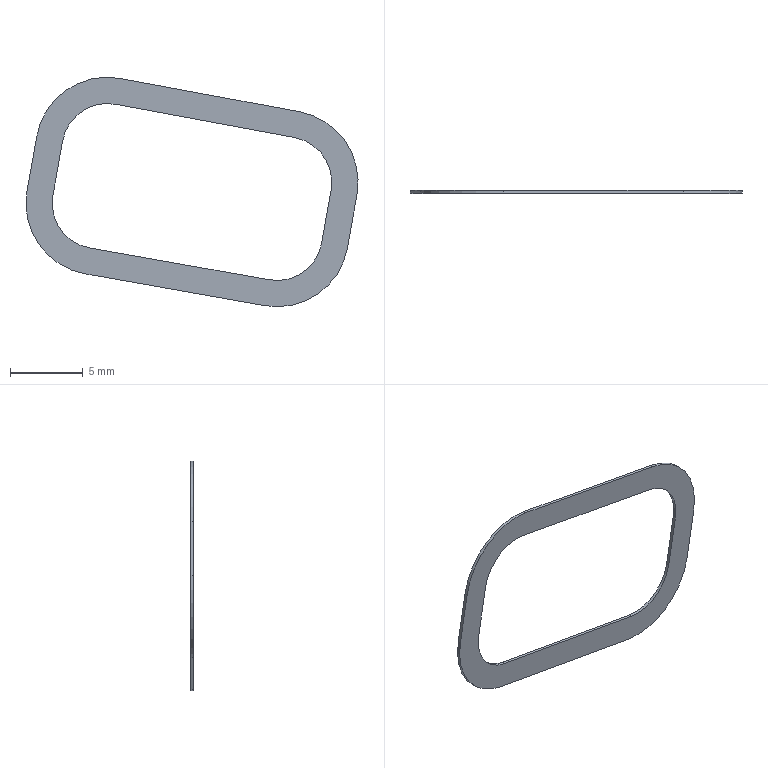Part | SolidWorks | features BaseBody 1 | 1 solid | 18 faces | box 22.755 x 0.2 x 15.726 mm | volume 20.749 mm3 | plane 10 | cylinder 8 | commonest cylinder face diameters 6.2 x4 9.8 x4
STEP:
#1=CARTESIAN_POINT('',(2027.605,-53.255,875.692));
#2=VERTEX_POINT('',#1);
#3=CARTESIAN_POINT('',(2027.605,-53.455,875.692));
#4=VERTEX_POINT('',#3);
#5=CARTESIAN_POINT('',(2027.605,-53.255,875.692));
#6=DIRECTION('',(0.,-1.,0.));
#7=VECTOR('',#6,1000.);
#8=LINE('',#5,#7);
#9=EDGE_CURVE('',#2,#4,#8,.T.);
#10=ORIENTED_EDGE('',*,*,#9,.T.);
#11=CARTESIAN_POINT('',(2033.303,-53.455,879.719));
#12=VERTEX_POINT('',#11);
#13=CARTESIAN_POINT('',(2032.44,-53.455,874.895));
#14=DIRECTION('',(0.,-1.,0.));
#15=DIRECTION('',(0.1761,0.,0.9844));
#16=AXIS2_PLACEMENT_3D('',#13,#14,#15);
#17=CIRCLE('',#16,4.9);
#18=EDGE_CURVE('',#12,#4,#17,.T.);
#19=ORIENTED_EDGE('',*,*,#18,.F.);
#20=CARTESIAN_POINT('',(2033.303,-53.255,879.719));
#21=VERTEX_POINT('',#20);
#22=CARTESIAN_POINT('',(2033.303,-53.255,879.719));
#23=DIRECTION('',(0.,-1.,0.));
#24=VECTOR('',#23,1000.);
#25=LINE('',#22,#24);
#26=EDGE_CURVE('',#21,#12,#25,.T.);
#27=ORIENTED_EDGE('',*,*,#26,.F.);
#28=CARTESIAN_POINT('',(2032.44,-53.255,874.895));
#29=DIRECTION('',(0.,-1.,0.));
#30=DIRECTION('',(0.1761,0.,0.9844));
#31=AXIS2_PLACEMENT_3D('',#28,#29,#30);
#32=CIRCLE('',#31,4.9);
#33=EDGE_CURVE('',#21,#2,#32,.T.);
#34=ORIENTED_EDGE('',*,*,#33,.T.);
#35=EDGE_LOOP('',(#10,#19,#27,#34));
#36=FACE_OUTER_BOUND('',#35,.T.);
#37=CARTESIAN_POINT('',(2032.44,-53.255,874.895));
#38=DIRECTION('',(0.,-1.,0.));
#39=DIRECTION('',(0.9846,0.,-0.1747));
#40=AXIS2_PLACEMENT_3D('',#37,#38,#39);
#41=CYLINDRICAL_SURFACE('',#40,4.9);
#42=ADVANCED_FACE('',(#36),#41,.T.);
#43=ORIENTED_EDGE('',*,*,#33,.F.);
#44=CARTESIAN_POINT('',(2045.593,-53.255,877.436));
#45=VERTEX_POINT('',#44);
#46=CARTESIAN_POINT('',(2045.593,-53.255,877.436));
#47=DIRECTION('',(-0.9832,0.,0.1826));
#48=VECTOR('',#47,1000.);
#49=LINE('',#46,#48);
#50=EDGE_CURVE('',#45,#21,#49,.T.);
#51=ORIENTED_EDGE('',*,*,#50,.F.);
#52=CARTESIAN_POINT('',(2049.566,-53.255,871.815));
#53=VERTEX_POINT('',#52);
#54=CARTESIAN_POINT('',(2044.731,-53.255,872.612));
#55=DIRECTION('',(0.,-1.,0.));
#56=DIRECTION('',(0.9867,0.,-0.1627));
#57=AXIS2_PLACEMENT_3D('',#54,#55,#56);
#58=CIRCLE('',#57,4.9);
#59=EDGE_CURVE('',#53,#45,#58,.T.);
#60=ORIENTED_EDGE('',*,*,#59,.F.);
#61=CARTESIAN_POINT('',(2048.898,-53.255,868.054));
#62=VERTEX_POINT('',#61);
#63=CARTESIAN_POINT('',(2048.898,-53.255,868.054));
#64=DIRECTION('',(0.1747,0.,0.9846));
#65=VECTOR('',#64,1000.);
#66=LINE('',#63,#65);
#67=EDGE_CURVE('',#62,#53,#66,.T.);
#68=ORIENTED_EDGE('',*,*,#67,.F.);
#69=CARTESIAN_POINT('',(2043.228,-53.255,864.144));
#70=VERTEX_POINT('',#69);
#71=CARTESIAN_POINT('',(2044.085,-53.255,868.969));
#72=DIRECTION('',(0.,-1.,0.));
#73=DIRECTION('',(-0.1747,0.,-0.9846));
#74=AXIS2_PLACEMENT_3D('',#71,#72,#73);
#75=CIRCLE('',#74,4.9);
#76=EDGE_CURVE('',#70,#62,#75,.T.);
#77=ORIENTED_EDGE('',*,*,#76,.F.);
#78=CARTESIAN_POINT('',(2030.92,-53.255,866.329));
#79=VERTEX_POINT('',#78);
#80=CARTESIAN_POINT('',(2030.92,-53.255,866.329));
#81=DIRECTION('',(0.9846,0.,-0.1747));
#82=VECTOR('',#81,1000.);
#83=LINE('',#80,#82);
#84=EDGE_CURVE('',#79,#70,#83,.T.);
#85=ORIENTED_EDGE('',*,*,#84,.F.);
#86=CARTESIAN_POINT('',(2026.941,-53.255,871.951));
#87=VERTEX_POINT('',#86);
#88=CARTESIAN_POINT('',(2031.776,-53.255,871.153));
#89=DIRECTION('',(0.,-1.,0.));
#90=DIRECTION('',(-0.9867,0.,0.1627));
#91=AXIS2_PLACEMENT_3D('',#88,#89,#90);
#92=CIRCLE('',#91,4.9);
#93=EDGE_CURVE('',#87,#79,#92,.T.);
#94=ORIENTED_EDGE('',*,*,#93,.F.);
#95=CARTESIAN_POINT('',(2027.605,-53.255,875.692));
#96=DIRECTION('',(-0.1747,0.,-0.9846));
#97=VECTOR('',#96,1000.);
#98=LINE('',#95,#97);
#99=EDGE_CURVE('',#2,#87,#98,.T.);
#100=ORIENTED_EDGE('',*,*,#99,.F.);
#101=EDGE_LOOP('',(#43,#51,#60,#68,#77,#85,#94,#100));
#102=FACE_OUTER_BOUND('',#101,.T.);
#103=CARTESIAN_POINT('',(2028.716,-53.255,871.648));
#104=VERTEX_POINT('',#103);
#105=CARTESIAN_POINT('',(2029.38,-53.255,875.39));
#106=VERTEX_POINT('',#105);
#107=CARTESIAN_POINT('',(2028.716,-53.255,871.648));
#108=DIRECTION('',(0.1747,0.,0.9846));
#109=VECTOR('',#108,1000.);
#110=LINE('',#107,#109);
#111=EDGE_CURVE('',#104,#106,#110,.T.);
#112=ORIENTED_EDGE('',*,*,#111,.F.);
#113=CARTESIAN_POINT('',(2031.235,-53.255,868.101));
#114=VERTEX_POINT('',#113);
#115=CARTESIAN_POINT('',(2031.776,-53.255,871.153));
#116=DIRECTION('',(0.,1.,0.));
#117=DIRECTION('',(-0.1746,0.,-0.9846));
#118=AXIS2_PLACEMENT_3D('',#115,#116,#117);
#119=CIRCLE('',#118,3.1);
#120=EDGE_CURVE('',#114,#104,#119,.T.);
#121=ORIENTED_EDGE('',*,*,#120,.F.);
#122=CARTESIAN_POINT('',(2043.543,-53.255,865.917));
#123=VERTEX_POINT('',#122);
#124=CARTESIAN_POINT('',(2043.543,-53.255,865.917));
#125=DIRECTION('',(-0.9846,0.,0.1747));
#126=VECTOR('',#125,1000.);
#127=LINE('',#124,#126);
#128=EDGE_CURVE('',#123,#114,#127,.T.);
#129=ORIENTED_EDGE('',*,*,#128,.F.);
#130=CARTESIAN_POINT('',(2047.128,-53.255,868.38));
#131=VERTEX_POINT('',#130);
#132=CARTESIAN_POINT('',(2044.085,-53.255,868.969));
#133=DIRECTION('',(0.,1.,0.));
#134=DIRECTION('',(0.9818,0.,-0.1899));
#135=AXIS2_PLACEMENT_3D('',#132,#133,#134);
#136=CIRCLE('',#135,3.1);
#137=EDGE_CURVE('',#131,#123,#136,.T.);
#138=ORIENTED_EDGE('',*,*,#137,.F.);
#139=CARTESIAN_POINT('',(2047.791,-53.255,872.117));
#140=VERTEX_POINT('',#139);
#141=CARTESIAN_POINT('',(2047.791,-53.255,872.117));
#142=DIRECTION('',(-0.1747,0.,-0.9846));
#143=VECTOR('',#142,1000.);
#144=LINE('',#141,#143);
#145=EDGE_CURVE('',#140,#131,#144,.T.);
#146=ORIENTED_EDGE('',*,*,#145,.F.);
#147=CARTESIAN_POINT('',(2045.271,-53.255,875.665));
#148=VERTEX_POINT('',#147);
#149=CARTESIAN_POINT('',(2044.731,-53.255,872.612));
#150=DIRECTION('',(0.,1.,0.));
#151=DIRECTION('',(0.1743,0.,0.9847));
#152=AXIS2_PLACEMENT_3D('',#149,#150,#151);
#153=CIRCLE('',#152,3.1);
#154=EDGE_CURVE('',#148,#140,#153,.T.);
#155=ORIENTED_EDGE('',*,*,#154,.F.);
#156=CARTESIAN_POINT('',(2032.981,-53.255,877.948));
#157=VERTEX_POINT('',#156);
#158=CARTESIAN_POINT('',(2032.981,-53.255,877.948));
#159=DIRECTION('',(0.9832,0.,-0.1826));
#160=VECTOR('',#159,1000.);
#161=LINE('',#158,#160);
#162=EDGE_CURVE('',#157,#148,#161,.T.);
#163=ORIENTED_EDGE('',*,*,#162,.F.);
#164=CARTESIAN_POINT('',(2032.44,-53.255,874.895));
#165=DIRECTION('',(0.,1.,0.));
#166=DIRECTION('',(-0.9872,0.,0.1595));
#167=AXIS2_PLACEMENT_3D('',#164,#165,#166);
#168=CIRCLE('',#167,3.1);
#169=EDGE_CURVE('',#106,#157,#168,.T.);
#170=ORIENTED_EDGE('',*,*,#169,.F.);
#171=EDGE_LOOP('',(#112,#121,#129,#138,#146,#155,#163,#170));
#172=FACE_BOUND('',#171,.T.);
#173=CARTESIAN_POINT('',(2032.4,-53.255,838.898));
#174=DIRECTION('',(0.,-1.,0.));
#175=DIRECTION('',(0.9846,0.,-0.1747));
#176=AXIS2_PLACEMENT_3D('',#173,#174,#175);
#177=PLANE('',#176);
#178=ADVANCED_FACE('',(#102,#172),#177,.F.);
#179=CARTESIAN_POINT('',(2032.981,-53.455,877.948));
#180=VERTEX_POINT('',#179);
#181=CARTESIAN_POINT('',(2032.981,-53.255,877.948));
#182=DIRECTION('',(0.,-1.,0.));
#183=VECTOR('',#182,1000.);
#184=LINE('',#181,#183);
#185=EDGE_CURVE('',#157,#180,#184,.T.);
#186=ORIENTED_EDGE('',*,*,#185,.T.);
#187=CARTESIAN_POINT('',(2029.38,-53.455,875.39));
#188=VERTEX_POINT('',#187);
#189=CARTESIAN_POINT('',(2032.44,-53.455,874.895));
#190=DIRECTION('',(0.,1.,0.));
#191=DIRECTION('',(-0.9872,0.,0.1595));
#192=AXIS2_PLACEMENT_3D('',#189,#190,#191);
#193=CIRCLE('',#192,3.1);
#194=EDGE_CURVE('',#188,#180,#193,.T.);
#195=ORIENTED_EDGE('',*,*,#194,.F.);
#196=CARTESIAN_POINT('',(2029.38,-53.255,875.39));
#197=DIRECTION('',(0.,-1.,0.));
#198=VECTOR('',#197,1000.);
#199=LINE('',#196,#198);
#200=EDGE_CURVE('',#106,#188,#199,.T.);
#201=ORIENTED_EDGE('',*,*,#200,.F.);
#202=ORIENTED_EDGE('',*,*,#169,.T.);
#203=EDGE_LOOP('',(#186,#195,#201,#202));
#204=FACE_OUTER_BOUND('',#203,.T.);
#205=CARTESIAN_POINT('',(2032.44,-53.255,874.895));
#206=DIRECTION('',(0.,-1.,0.));
#207=DIRECTION('',(0.9846,0.,-0.1747));
#208=AXIS2_PLACEMENT_3D('',#205,#206,#207);
#209=CYLINDRICAL_SURFACE('',#208,3.1);
#210=ADVANCED_FACE('',(#204),#209,.F.);
#211=ORIENTED_EDGE('',*,*,#200,.T.);
#212=CARTESIAN_POINT('',(2028.716,-53.455,871.648));
#213=VERTEX_POINT('',#212);
#214=CARTESIAN_POINT('',(2028.716,-53.455,871.648));
#215=DIRECTION('',(0.1747,0.,0.9846));
#216=VECTOR('',#215,1000.);
#217=LINE('',#214,#216);
#218=EDGE_CURVE('',#213,#188,#217,.T.);
#219=ORIENTED_EDGE('',*,*,#218,.F.);
#220=CARTESIAN_POINT('',(2028.716,-53.255,871.648));
#221=DIRECTION('',(0.,-1.,0.));
#222=VECTOR('',#221,1000.);
#223=LINE('',#220,#222);
#224=EDGE_CURVE('',#104,#213,#223,.T.);
#225=ORIENTED_EDGE('',*,*,#224,.F.);
#226=ORIENTED_EDGE('',*,*,#111,.T.);
#227=EDGE_LOOP('',(#211,#219,#225,#226));
#228=FACE_OUTER_BOUND('',#227,.T.);
#229=CARTESIAN_POINT('',(2028.716,-53.255,871.648));
#230=DIRECTION('',(0.9846,0.,-0.1747));
#231=DIRECTION('',(-0.1747,0.,-0.9846));
#232=AXIS2_PLACEMENT_3D('',#229,#230,#231);
#233=PLANE('',#232);
#234=ADVANCED_FACE('',(#228),#233,.T.);
#235=ORIENTED_EDGE('',*,*,#224,.T.);
#236=CARTESIAN_POINT('',(2031.235,-53.455,868.101));
#237=VERTEX_POINT('',#236);
#238=CARTESIAN_POINT('',(2031.776,-53.455,871.153));
#239=DIRECTION('',(0.,1.,0.));
#240=DIRECTION('',(-0.1746,0.,-0.9846));
#241=AXIS2_PLACEMENT_3D('',#238,#239,#240);
#242=CIRCLE('',#241,3.1);
#243=EDGE_CURVE('',#237,#213,#242,.T.);
#244=ORIENTED_EDGE('',*,*,#243,.F.);
#245=CARTESIAN_POINT('',(2031.235,-53.255,868.101));
#246=DIRECTION('',(0.,-1.,0.));
#247=VECTOR('',#246,1000.);
#248=LINE('',#245,#247);
#249=EDGE_CURVE('',#114,#237,#248,.T.);
#250=ORIENTED_EDGE('',*,*,#249,.F.);
#251=ORIENTED_EDGE('',*,*,#120,.T.);
#252=EDGE_LOOP('',(#235,#244,#250,#251));
#253=FACE_OUTER_BOUND('',#252,.T.);
#254=CARTESIAN_POINT('',(2031.776,-53.255,871.153));
#255=DIRECTION('',(0.,-1.,0.));
#256=DIRECTION('',(0.9846,0.,-0.1747));
#257=AXIS2_PLACEMENT_3D('',#254,#255,#256);
#258=CYLINDRICAL_SURFACE('',#257,3.1);
#259=ADVANCED_FACE('',(#253),#258,.F.);
#260=ORIENTED_EDGE('',*,*,#249,.T.);
#261=CARTESIAN_POINT('',(2043.543,-53.455,865.917));
#262=VERTEX_POINT('',#261);
#263=CARTESIAN_POINT('',(2043.543,-53.455,865.917));
#264=DIRECTION('',(-0.9846,0.,0.1747));
#265=VECTOR('',#264,1000.);
#266=LINE('',#263,#265);
#267=EDGE_CURVE('',#262,#237,#266,.T.);
#268=ORIENTED_EDGE('',*,*,#267,.F.);
#269=CARTESIAN_POINT('',(2043.543,-53.255,865.917));
#270=DIRECTION('',(0.,-1.,0.));
#271=VECTOR('',#270,1000.);
#272=LINE('',#269,#271);
#273=EDGE_CURVE('',#123,#262,#272,.T.);
#274=ORIENTED_EDGE('',*,*,#273,.F.);
#275=ORIENTED_EDGE('',*,*,#128,.T.);
#276=EDGE_LOOP('',(#260,#268,#274,#275));
#277=FACE_OUTER_BOUND('',#276,.T.);
#278=CARTESIAN_POINT('',(2043.543,-53.255,865.917));
#279=DIRECTION('',(0.1747,0.,0.9846));
#280=DIRECTION('',(0.9846,0.,-0.1747));
#281=AXIS2_PLACEMENT_3D('',#278,#279,#280);
#282=PLANE('',#281);
#283=ADVANCED_FACE('',(#277),#282,.T.);
#284=ORIENTED_EDGE('',*,*,#273,.T.);
#285=CARTESIAN_POINT('',(2047.128,-53.455,868.38));
#286=VERTEX_POINT('',#285);
#287=CARTESIAN_POINT('',(2044.085,-53.455,868.969));
#288=DIRECTION('',(0.,1.,0.));
#289=DIRECTION('',(0.9818,0.,-0.1899));
#290=AXIS2_PLACEMENT_3D('',#287,#288,#289);
#291=CIRCLE('',#290,3.1);
#292=EDGE_CURVE('',#286,#262,#291,.T.);
#293=ORIENTED_EDGE('',*,*,#292,.F.);
#294=CARTESIAN_POINT('',(2047.128,-53.255,868.38));
#295=DIRECTION('',(0.,-1.,0.));
#296=VECTOR('',#295,1000.);
#297=LINE('',#294,#296);
#298=EDGE_CURVE('',#131,#286,#297,.T.);
#299=ORIENTED_EDGE('',*,*,#298,.F.);
#300=ORIENTED_EDGE('',*,*,#137,.T.);
#301=EDGE_LOOP('',(#284,#293,#299,#300));
#302=FACE_OUTER_BOUND('',#301,.T.);
#303=CARTESIAN_POINT('',(2044.085,-53.255,868.969));
#304=DIRECTION('',(0.,-1.,0.));
#305=DIRECTION('',(0.9846,0.,-0.1747));
#306=AXIS2_PLACEMENT_3D('',#303,#304,#305);
#307=CYLINDRICAL_SURFACE('',#306,3.1);
#308=ADVANCED_FACE('',(#302),#307,.F.);
#309=ORIENTED_EDGE('',*,*,#298,.T.);
#310=CARTESIAN_POINT('',(2047.791,-53.455,872.117));
#311=VERTEX_POINT('',#310);
#312=CARTESIAN_POINT('',(2047.791,-53.455,872.117));
#313=DIRECTION('',(-0.1747,0.,-0.9846));
#314=VECTOR('',#313,1000.);
#315=LINE('',#312,#314);
#316=EDGE_CURVE('',#311,#286,#315,.T.);
#317=ORIENTED_EDGE('',*,*,#316,.F.);
#318=CARTESIAN_POINT('',(2047.791,-53.255,872.117));
#319=DIRECTION('',(0.,-1.,0.));
#320=VECTOR('',#319,1000.);
#321=LINE('',#318,#320);
#322=EDGE_CURVE('',#140,#311,#321,.T.);
#323=ORIENTED_EDGE('',*,*,#322,.F.);
#324=ORIENTED_EDGE('',*,*,#145,.T.);
#325=EDGE_LOOP('',(#309,#317,#323,#324));
#326=FACE_OUTER_BOUND('',#325,.T.);
#327=CARTESIAN_POINT('',(2047.791,-53.255,872.117));
#328=DIRECTION('',(-0.9846,0.,0.1747));
#329=DIRECTION('',(0.1747,0.,0.9846));
#330=AXIS2_PLACEMENT_3D('',#327,#328,#329);
#331=PLANE('',#330);
#332=ADVANCED_FACE('',(#326),#331,.T.);
#333=ORIENTED_EDGE('',*,*,#322,.T.);
#334=CARTESIAN_POINT('',(2045.271,-53.455,875.665));
#335=VERTEX_POINT('',#334);
#336=CARTESIAN_POINT('',(2044.731,-53.455,872.612));
#337=DIRECTION('',(0.,1.,0.));
#338=DIRECTION('',(0.1743,0.,0.9847));
#339=AXIS2_PLACEMENT_3D('',#336,#337,#338);
#340=CIRCLE('',#339,3.1);
#341=EDGE_CURVE('',#335,#311,#340,.T.);
#342=ORIENTED_EDGE('',*,*,#341,.F.);
#343=CARTESIAN_POINT('',(2045.271,-53.255,875.665));
#344=DIRECTION('',(0.,-1.,0.));
#345=VECTOR('',#344,1000.);
#346=LINE('',#343,#345);
#347=EDGE_CURVE('',#148,#335,#346,.T.);
#348=ORIENTED_EDGE('',*,*,#347,.F.);
#349=ORIENTED_EDGE('',*,*,#154,.T.);
#350=EDGE_LOOP('',(#333,#342,#348,#349));
#351=FACE_OUTER_BOUND('',#350,.T.);
#352=CARTESIAN_POINT('',(2044.731,-53.255,872.612));
#353=DIRECTION('',(0.,-1.,0.));
#354=DIRECTION('',(0.9846,0.,-0.1747));
#355=AXIS2_PLACEMENT_3D('',#352,#353,#354);
#356=CYLINDRICAL_SURFACE('',#355,3.1);
#357=ADVANCED_FACE('',(#351),#356,.F.);
#358=ORIENTED_EDGE('',*,*,#347,.T.);
#359=CARTESIAN_POINT('',(2032.981,-53.455,877.948));
#360=DIRECTION('',(0.9832,0.,-0.1826));
#361=VECTOR('',#360,1000.);
#362=LINE('',#359,#361);
#363=EDGE_CURVE('',#180,#335,#362,.T.);
#364=ORIENTED_EDGE('',*,*,#363,.F.);
#365=ORIENTED_EDGE('',*,*,#185,.F.);
#366=ORIENTED_EDGE('',*,*,#162,.T.);
#367=EDGE_LOOP('',(#358,#364,#365,#366));
#368=FACE_OUTER_BOUND('',#367,.T.);
#369=CARTESIAN_POINT('',(2032.981,-53.255,877.948));
#370=DIRECTION('',(-0.1826,0.,-0.9832));
#371=DIRECTION('',(-0.9832,0.,0.1826));
#372=AXIS2_PLACEMENT_3D('',#369,#370,#371);
#373=PLANE('',#372);
#374=ADVANCED_FACE('',(#368),#373,.T.);
#375=CARTESIAN_POINT('',(2026.941,-53.455,871.951));
#376=VERTEX_POINT('',#375);
#377=CARTESIAN_POINT('',(2030.92,-53.455,866.329));
#378=VERTEX_POINT('',#377);
#379=CARTESIAN_POINT('',(2031.776,-53.455,871.153));
#380=DIRECTION('',(0.,-1.,0.));
#381=DIRECTION('',(-0.9867,0.,0.1627));
#382=AXIS2_PLACEMENT_3D('',#379,#380,#381);
#383=CIRCLE('',#382,4.9);
#384=EDGE_CURVE('',#376,#378,#383,.T.);
#385=ORIENTED_EDGE('',*,*,#384,.T.);
#386=CARTESIAN_POINT('',(2043.228,-53.455,864.144));
#387=VERTEX_POINT('',#386);
#388=CARTESIAN_POINT('',(2030.92,-53.455,866.329));
#389=DIRECTION('',(0.9846,0.,-0.1747));
#390=VECTOR('',#389,1000.);
#391=LINE('',#388,#390);
#392=EDGE_CURVE('',#378,#387,#391,.T.);
#393=ORIENTED_EDGE('',*,*,#392,.T.);
#394=CARTESIAN_POINT('',(2048.898,-53.455,868.054));
#395=VERTEX_POINT('',#394);
#396=CARTESIAN_POINT('',(2044.085,-53.455,868.969));
#397=DIRECTION('',(0.,-1.,0.));
#398=DIRECTION('',(-0.1747,0.,-0.9846));
#399=AXIS2_PLACEMENT_3D('',#396,#397,#398);
#400=CIRCLE('',#399,4.9);
#401=EDGE_CURVE('',#387,#395,#400,.T.);
#402=ORIENTED_EDGE('',*,*,#401,.T.);
#403=CARTESIAN_POINT('',(2049.566,-53.455,871.815));
#404=VERTEX_POINT('',#403);
#405=CARTESIAN_POINT('',(2048.898,-53.455,868.054));
#406=DIRECTION('',(0.1747,0.,0.9846));
#407=VECTOR('',#406,1000.);
#408=LINE('',#405,#407);
#409=EDGE_CURVE('',#395,#404,#408,.T.);
#410=ORIENTED_EDGE('',*,*,#409,.T.);
#411=CARTESIAN_POINT('',(2045.593,-53.455,877.436));
#412=VERTEX_POINT('',#411);
#413=CARTESIAN_POINT('',(2044.731,-53.455,872.612));
#414=DIRECTION('',(0.,-1.,0.));
#415=DIRECTION('',(0.9867,0.,-0.1627));
#416=AXIS2_PLACEMENT_3D('',#413,#414,#415);
#417=CIRCLE('',#416,4.9);
#418=EDGE_CURVE('',#404,#412,#417,.T.);
#419=ORIENTED_EDGE('',*,*,#418,.T.);
#420=CARTESIAN_POINT('',(2045.593,-53.455,877.436));
#421=DIRECTION('',(-0.9832,0.,0.1826));
#422=VECTOR('',#421,1000.);
#423=LINE('',#420,#422);
#424=EDGE_CURVE('',#412,#12,#423,.T.);
#425=ORIENTED_EDGE('',*,*,#424,.T.);
#426=ORIENTED_EDGE('',*,*,#18,.T.);
#427=CARTESIAN_POINT('',(2027.605,-53.455,875.692));
#428=DIRECTION('',(-0.1747,0.,-0.9846));
#429=VECTOR('',#428,1000.);
#430=LINE('',#427,#429);
#431=EDGE_CURVE('',#4,#376,#430,.T.);
#432=ORIENTED_EDGE('',*,*,#431,.T.);
#433=EDGE_LOOP('',(#385,#393,#402,#410,#419,#425,#426,#432));
#434=FACE_OUTER_BOUND('',#433,.T.);
#435=ORIENTED_EDGE('',*,*,#363,.T.);
#436=ORIENTED_EDGE('',*,*,#341,.T.);
#437=ORIENTED_EDGE('',*,*,#316,.T.);
#438=ORIENTED_EDGE('',*,*,#292,.T.);
#439=ORIENTED_EDGE('',*,*,#267,.T.);
#440=ORIENTED_EDGE('',*,*,#243,.T.);
#441=ORIENTED_EDGE('',*,*,#218,.T.);
#442=ORIENTED_EDGE('',*,*,#194,.T.);
#443=EDGE_LOOP('',(#435,#436,#437,#438,#439,#440,#441,#442));
#444=FACE_BOUND('',#443,.T.);
#445=CARTESIAN_POINT('',(2032.4,-53.455,838.898));
#446=DIRECTION('',(0.,-1.,0.));
#447=DIRECTION('',(0.9846,0.,-0.1747));
#448=AXIS2_PLACEMENT_3D('',#445,#446,#447);
#449=PLANE('',#448);
#450=ADVANCED_FACE('',(#434,#444),#449,.T.);
#451=CARTESIAN_POINT('',(2026.941,-53.255,871.951));
#452=DIRECTION('',(0.,-1.,0.));
#453=VECTOR('',#452,1000.);
#454=LINE('',#451,#453);
#455=EDGE_CURVE('',#87,#376,#454,.T.);
#456=ORIENTED_EDGE('',*,*,#455,.T.);
#457=ORIENTED_EDGE('',*,*,#431,.F.);
#458=ORIENTED_EDGE('',*,*,#9,.F.);
#459=ORIENTED_EDGE('',*,*,#99,.T.);
#460=EDGE_LOOP('',(#456,#457,#458,#459));
#461=FACE_OUTER_BOUND('',#460,.T.);
#462=CARTESIAN_POINT('',(2027.605,-53.255,875.692));
#463=DIRECTION('',(-0.9846,0.,0.1747));
#464=DIRECTION('',(0.1747,0.,0.9846));
#465=AXIS2_PLACEMENT_3D('',#462,#463,#464);
#466=PLANE('',#465);
#467=ADVANCED_FACE('',(#461),#466,.T.);
#468=CARTESIAN_POINT('',(2030.92,-53.255,866.329));
#469=DIRECTION('',(0.,-1.,0.));
#470=VECTOR('',#469,1000.);
#471=LINE('',#468,#470);
#472=EDGE_CURVE('',#79,#378,#471,.T.);
#473=ORIENTED_EDGE('',*,*,#472,.T.);
#474=ORIENTED_EDGE('',*,*,#384,.F.);
#475=ORIENTED_EDGE('',*,*,#455,.F.);
#476=ORIENTED_EDGE('',*,*,#93,.T.);
#477=EDGE_LOOP('',(#473,#474,#475,#476));
#478=FACE_OUTER_BOUND('',#477,.T.);
#479=CARTESIAN_POINT('',(2031.776,-53.255,871.153));
#480=DIRECTION('',(0.,-1.,0.));
#481=DIRECTION('',(0.9846,0.,-0.1747));
#482=AXIS2_PLACEMENT_3D('',#479,#480,#481);
#483=CYLINDRICAL_SURFACE('',#482,4.9);
#484=ADVANCED_FACE('',(#478),#483,.T.);
#485=CARTESIAN_POINT('',(2043.228,-53.255,864.144));
#486=DIRECTION('',(0.,-1.,0.));
#487=VECTOR('',#486,1000.);
#488=LINE('',#485,#487);
#489=EDGE_CURVE('',#70,#387,#488,.T.);
#490=ORIENTED_EDGE('',*,*,#489,.T.);
#491=ORIENTED_EDGE('',*,*,#392,.F.);
#492=ORIENTED_EDGE('',*,*,#472,.F.);
#493=ORIENTED_EDGE('',*,*,#84,.T.);
#494=EDGE_LOOP('',(#490,#491,#492,#493));
#495=FACE_OUTER_BOUND('',#494,.T.);
#496=CARTESIAN_POINT('',(2030.92,-53.255,866.329));
#497=DIRECTION('',(-0.1747,0.,-0.9846));
#498=DIRECTION('',(-0.9846,0.,0.1747));
#499=AXIS2_PLACEMENT_3D('',#496,#497,#498);
#500=PLANE('',#499);
#501=ADVANCED_FACE('',(#495),#500,.T.);
#502=CARTESIAN_POINT('',(2048.898,-53.255,868.054));
#503=DIRECTION('',(0.,-1.,0.));
#504=VECTOR('',#503,1000.);
#505=LINE('',#502,#504);
#506=EDGE_CURVE('',#62,#395,#505,.T.);
#507=ORIENTED_EDGE('',*,*,#506,.T.);
#508=ORIENTED_EDGE('',*,*,#401,.F.);
#509=ORIENTED_EDGE('',*,*,#489,.F.);
#510=ORIENTED_EDGE('',*,*,#76,.T.);
#511=EDGE_LOOP('',(#507,#508,#509,#510));
#512=FACE_OUTER_BOUND('',#511,.T.);
#513=CARTESIAN_POINT('',(2044.085,-53.255,868.969));
#514=DIRECTION('',(0.,-1.,0.));
#515=DIRECTION('',(0.9846,0.,-0.1747));
#516=AXIS2_PLACEMENT_3D('',#513,#514,#515);
#517=CYLINDRICAL_SURFACE('',#516,4.9);
#518=ADVANCED_FACE('',(#512),#517,.T.);
#519=CARTESIAN_POINT('',(2049.566,-53.255,871.815));
#520=DIRECTION('',(0.,-1.,0.));
#521=VECTOR('',#520,1000.);
#522=LINE('',#519,#521);
#523=EDGE_CURVE('',#53,#404,#522,.T.);
#524=ORIENTED_EDGE('',*,*,#523,.T.);
#525=ORIENTED_EDGE('',*,*,#409,.F.);
#526=ORIENTED_EDGE('',*,*,#506,.F.);
#527=ORIENTED_EDGE('',*,*,#67,.T.);
#528=EDGE_LOOP('',(#524,#525,#526,#527));
#529=FACE_OUTER_BOUND('',#528,.T.);
#530=CARTESIAN_POINT('',(2048.898,-53.255,868.054));
#531=DIRECTION('',(0.9846,0.,-0.1747));
#532=DIRECTION('',(-0.1747,0.,-0.9846));
#533=AXIS2_PLACEMENT_3D('',#530,#531,#532);
#534=PLANE('',#533);
#535=ADVANCED_FACE('',(#529),#534,.T.);
#536=CARTESIAN_POINT('',(2045.593,-53.255,877.436));
#537=DIRECTION('',(0.,-1.,0.));
#538=VECTOR('',#537,1000.);
#539=LINE('',#536,#538);
#540=EDGE_CURVE('',#45,#412,#539,.T.);
#541=ORIENTED_EDGE('',*,*,#540,.T.);
#542=ORIENTED_EDGE('',*,*,#418,.F.);
#543=ORIENTED_EDGE('',*,*,#523,.F.);
#544=ORIENTED_EDGE('',*,*,#59,.T.);
#545=EDGE_LOOP('',(#541,#542,#543,#544));
#546=FACE_OUTER_BOUND('',#545,.T.);
#547=CARTESIAN_POINT('',(2044.731,-53.255,872.612));
#548=DIRECTION('',(0.,-1.,0.));
#549=DIRECTION('',(0.9846,0.,-0.1747));
#550=AXIS2_PLACEMENT_3D('',#547,#548,#549);
#551=CYLINDRICAL_SURFACE('',#550,4.9);
#552=ADVANCED_FACE('',(#546),#551,.T.);
#553=ORIENTED_EDGE('',*,*,#26,.T.);
#554=ORIENTED_EDGE('',*,*,#424,.F.);
#555=ORIENTED_EDGE('',*,*,#540,.F.);
#556=ORIENTED_EDGE('',*,*,#50,.T.);
#557=EDGE_LOOP('',(#553,#554,#555,#556));
#558=FACE_OUTER_BOUND('',#557,.T.);
#559=CARTESIAN_POINT('',(2045.593,-53.255,877.436));
#560=DIRECTION('',(0.1826,0.,0.9832));
#561=DIRECTION('',(0.9832,0.,-0.1826));
#562=AXIS2_PLACEMENT_3D('',#559,#560,#561);
#563=PLANE('',#562);
#564=ADVANCED_FACE('',(#558),#563,.T.);
#565=CLOSED_SHELL('',(#42,#178,#210,#234,#259,#283,#308,#332,#357,#374,#450,#467,#484,#501,#518,#535,#552,#564));
#566=MANIFOLD_SOLID_BREP('',#565);
#567=CARTESIAN_POINT('',(0.,0.,0.));
#568=DIRECTION('',(0.,0.,1.));
#569=DIRECTION('',(1.,0.,0.));
#570=AXIS2_PLACEMENT_3D('',#567,#568,#569);
#571=(LENGTH_UNIT()NAMED_UNIT(*)SI_UNIT(.MILLI.,.METRE.));
#572=UNCERTAINTY_MEASURE_WITH_UNIT(LENGTH_MEASURE(0.00001),#571,'','');
#573=(NAMED_UNIT(*)PLANE_ANGLE_UNIT()SI_UNIT($,.RADIAN.));
#574=(NAMED_UNIT(*)SI_UNIT($,.STERADIAN.)SOLID_ANGLE_UNIT());
#575=(GEOMETRIC_REPRESENTATION_CONTEXT(3)GLOBAL_UNCERTAINTY_ASSIGNED_CONTEXT((#572))GLOBAL_UNIT_ASSIGNED_CONTEXT((#571,#573,#574))REPRESENTATION_CONTEXT('',''));
#576=ADVANCED_BREP_SHAPE_REPRESENTATION('',(#566,#570),#575);